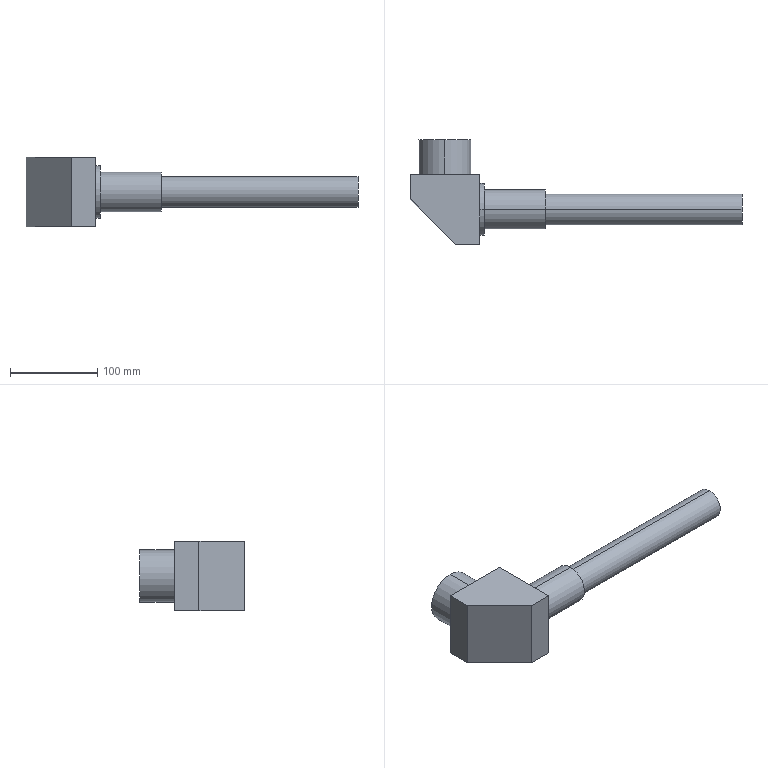Part | NX | features BREP 1 | 1 solid | 19 faces | box 380 x 120 x 80 mm | volume 858880 mm3 | plane 11 | cylinder 8 | commonest cylinder face diameters 60 x4 35 x2 45 x2
STEP:
#1=CARTESIAN_POINT('',(380.,-40.,22.5));
#2=VERTEX_POINT('',#1);
#3=CARTESIAN_POINT('',(380.,-40.,57.5));
#4=VERTEX_POINT('',#3);
#5=CARTESIAN_POINT('',(380.,-40.,40.));
#6=DIRECTION('',(1.,0.,0.));
#7=DIRECTION('',(0.,0.,-1.));
#8=AXIS2_PLACEMENT_3D('',#5,#6,#7);
#9=CIRCLE('',#8,17.5);
#10=EDGE_CURVE('',#2,#4,#9,.T.);
#11=ORIENTED_EDGE('',*,*,#10,.F.);
#12=CARTESIAN_POINT('',(155.,-40.,22.5));
#13=VERTEX_POINT('',#12);
#14=CARTESIAN_POINT('',(380.,-40.,22.5));
#15=DIRECTION('',(-1.,0.,0.));
#16=VECTOR('',#15,1000.);
#17=LINE('',#14,#16);
#18=EDGE_CURVE('',#13,#2,#17,.F.);
#19=ORIENTED_EDGE('',*,*,#18,.F.);
#20=CARTESIAN_POINT('',(155.,-40.,57.5));
#21=VERTEX_POINT('',#20);
#22=CARTESIAN_POINT('',(155.,-40.,40.));
#23=DIRECTION('',(1.,0.,0.));
#24=DIRECTION('',(0.,0.,-1.));
#25=AXIS2_PLACEMENT_3D('',#22,#23,#24);
#26=CIRCLE('',#25,17.5);
#27=EDGE_CURVE('',#13,#21,#26,.T.);
#28=ORIENTED_EDGE('',*,*,#27,.T.);
#29=CARTESIAN_POINT('',(380.,-40.,57.5));
#30=DIRECTION('',(-1.,0.,0.));
#31=VECTOR('',#30,1000.);
#32=LINE('',#29,#31);
#33=EDGE_CURVE('',#21,#4,#32,.F.);
#34=ORIENTED_EDGE('',*,*,#33,.T.);
#35=EDGE_LOOP('',(#11,#19,#28,#34));
#36=FACE_BOUND('',#35,.T.);
#37=CARTESIAN_POINT('',(380.,-40.,40.));
#38=DIRECTION('',(-1.,0.,0.));
#39=DIRECTION('',(0.,0.,1.));
#40=AXIS2_PLACEMENT_3D('',#37,#38,#39);
#41=CYLINDRICAL_SURFACE('',#40,17.5);
#42=ADVANCED_FACE('',(#36),#41,.T.);
#43=CARTESIAN_POINT('',(40.,40.,70.));
#44=VERTEX_POINT('',#43);
#45=CARTESIAN_POINT('',(40.,40.,10.));
#46=VERTEX_POINT('',#45);
#47=CARTESIAN_POINT('',(40.,40.,40.));
#48=DIRECTION('',(0.,1.,0.));
#49=DIRECTION('',(0.,0.,1.));
#50=AXIS2_PLACEMENT_3D('',#47,#48,#49);
#51=CIRCLE('',#50,30.);
#52=EDGE_CURVE('',#44,#46,#51,.T.);
#53=ORIENTED_EDGE('',*,*,#52,.F.);
#54=CARTESIAN_POINT('',(40.,0.,70.));
#55=VERTEX_POINT('',#54);
#56=CARTESIAN_POINT('',(40.,40.,70.));
#57=DIRECTION('',(0.,-1.,0.));
#58=VECTOR('',#57,1000.);
#59=LINE('',#56,#58);
#60=EDGE_CURVE('',#44,#55,#59,.T.);
#61=ORIENTED_EDGE('',*,*,#60,.T.);
#62=CARTESIAN_POINT('',(40.,0.,10.));
#63=VERTEX_POINT('',#62);
#64=CARTESIAN_POINT('',(40.,0.,40.));
#65=DIRECTION('',(0.,1.,0.));
#66=DIRECTION('',(0.,0.,1.));
#67=AXIS2_PLACEMENT_3D('',#64,#65,#66);
#68=CIRCLE('',#67,30.);
#69=EDGE_CURVE('',#55,#63,#68,.T.);
#70=ORIENTED_EDGE('',*,*,#69,.T.);
#71=CARTESIAN_POINT('',(40.,40.,10.));
#72=DIRECTION('',(0.,-1.,0.));
#73=VECTOR('',#72,1000.);
#74=LINE('',#71,#73);
#75=EDGE_CURVE('',#46,#63,#74,.T.);
#76=ORIENTED_EDGE('',*,*,#75,.F.);
#77=EDGE_LOOP('',(#53,#61,#70,#76));
#78=FACE_BOUND('',#77,.T.);
#79=CARTESIAN_POINT('',(40.,40.,40.));
#80=DIRECTION('',(0.,-1.,0.));
#81=DIRECTION('',(0.,0.,-1.));
#82=AXIS2_PLACEMENT_3D('',#79,#80,#81);
#83=CYLINDRICAL_SURFACE('',#82,30.);
#84=ADVANCED_FACE('',(#78),#83,.T.);
#85=CARTESIAN_POINT('',(155.,-40.,17.5));
#86=VERTEX_POINT('',#85);
#87=CARTESIAN_POINT('',(155.,-40.,62.5));
#88=VERTEX_POINT('',#87);
#89=CARTESIAN_POINT('',(155.,-40.,40.));
#90=DIRECTION('',(1.,0.,0.));
#91=DIRECTION('',(0.,0.,-1.));
#92=AXIS2_PLACEMENT_3D('',#89,#90,#91);
#93=CIRCLE('',#92,22.5);
#94=EDGE_CURVE('',#86,#88,#93,.T.);
#95=ORIENTED_EDGE('',*,*,#94,.F.);
#96=CARTESIAN_POINT('',(85.,-40.,17.5));
#97=VERTEX_POINT('',#96);
#98=CARTESIAN_POINT('',(155.,-40.,17.5));
#99=DIRECTION('',(-1.,0.,0.));
#100=VECTOR('',#99,1000.);
#101=LINE('',#98,#100);
#102=EDGE_CURVE('',#97,#86,#101,.F.);
#103=ORIENTED_EDGE('',*,*,#102,.F.);
#104=CARTESIAN_POINT('',(85.,-40.,62.5));
#105=VERTEX_POINT('',#104);
#106=CARTESIAN_POINT('',(85.,-40.,40.));
#107=DIRECTION('',(1.,0.,0.));
#108=DIRECTION('',(0.,0.,-1.));
#109=AXIS2_PLACEMENT_3D('',#106,#107,#108);
#110=CIRCLE('',#109,22.5);
#111=EDGE_CURVE('',#97,#105,#110,.T.);
#112=ORIENTED_EDGE('',*,*,#111,.T.);
#113=CARTESIAN_POINT('',(155.,-40.,62.5));
#114=DIRECTION('',(-1.,0.,0.));
#115=VECTOR('',#114,1000.);
#116=LINE('',#113,#115);
#117=EDGE_CURVE('',#105,#88,#116,.F.);
#118=ORIENTED_EDGE('',*,*,#117,.T.);
#119=EDGE_LOOP('',(#95,#103,#112,#118));
#120=FACE_BOUND('',#119,.T.);
#121=CARTESIAN_POINT('',(155.,-40.,40.));
#122=DIRECTION('',(-1.,0.,0.));
#123=DIRECTION('',(0.,0.,1.));
#124=AXIS2_PLACEMENT_3D('',#121,#122,#123);
#125=CYLINDRICAL_SURFACE('',#124,22.5);
#126=ADVANCED_FACE('',(#120),#125,.T.);
#127=CARTESIAN_POINT('',(85.,-40.,10.));
#128=VERTEX_POINT('',#127);
#129=CARTESIAN_POINT('',(85.,-40.,70.));
#130=VERTEX_POINT('',#129);
#131=CARTESIAN_POINT('',(85.,-40.,40.));
#132=DIRECTION('',(1.,0.,0.));
#133=DIRECTION('',(0.,0.,-1.));
#134=AXIS2_PLACEMENT_3D('',#131,#132,#133);
#135=CIRCLE('',#134,30.);
#136=EDGE_CURVE('',#128,#130,#135,.T.);
#137=ORIENTED_EDGE('',*,*,#136,.F.);
#138=CARTESIAN_POINT('',(80.,-40.,10.));
#139=VERTEX_POINT('',#138);
#140=CARTESIAN_POINT('',(85.,-40.,10.));
#141=DIRECTION('',(-1.,0.,0.));
#142=VECTOR('',#141,1000.);
#143=LINE('',#140,#142);
#144=EDGE_CURVE('',#139,#128,#143,.F.);
#145=ORIENTED_EDGE('',*,*,#144,.F.);
#146=CARTESIAN_POINT('',(80.,-40.,70.));
#147=VERTEX_POINT('',#146);
#148=CARTESIAN_POINT('',(80.,-40.,40.));
#149=DIRECTION('',(1.,0.,0.));
#150=DIRECTION('',(0.,0.,-1.));
#151=AXIS2_PLACEMENT_3D('',#148,#149,#150);
#152=CIRCLE('',#151,30.);
#153=EDGE_CURVE('',#139,#147,#152,.T.);
#154=ORIENTED_EDGE('',*,*,#153,.T.);
#155=CARTESIAN_POINT('',(85.,-40.,70.));
#156=DIRECTION('',(-1.,0.,0.));
#157=VECTOR('',#156,1000.);
#158=LINE('',#155,#157);
#159=EDGE_CURVE('',#147,#130,#158,.F.);
#160=ORIENTED_EDGE('',*,*,#159,.T.);
#161=EDGE_LOOP('',(#137,#145,#154,#160));
#162=FACE_BOUND('',#161,.T.);
#163=CARTESIAN_POINT('',(85.,-40.,40.));
#164=DIRECTION('',(-1.,0.,0.));
#165=DIRECTION('',(0.,0.,1.));
#166=AXIS2_PLACEMENT_3D('',#163,#164,#165);
#167=CYLINDRICAL_SURFACE('',#166,30.);
#168=ADVANCED_FACE('',(#162),#167,.T.);
#169=CARTESIAN_POINT('',(0.,0.,0.));
#170=VERTEX_POINT('',#169);
#171=CARTESIAN_POINT('',(0.,-28.,0.));
#172=VERTEX_POINT('',#171);
#173=CARTESIAN_POINT('',(0.,-28.,0.));
#174=DIRECTION('',(0.,-1.,0.));
#175=VECTOR('',#174,1000.);
#176=LINE('',#173,#175);
#177=EDGE_CURVE('',#170,#172,#176,.T.);
#178=ORIENTED_EDGE('',*,*,#177,.T.);
#179=CARTESIAN_POINT('',(0.,-28.,80.));
#180=VERTEX_POINT('',#179);
#181=CARTESIAN_POINT('',(0.,-28.,80.));
#182=DIRECTION('',(0.,0.,-1.));
#183=VECTOR('',#182,1000.);
#184=LINE('',#181,#183);
#185=EDGE_CURVE('',#180,#172,#184,.T.);
#186=ORIENTED_EDGE('',*,*,#185,.F.);
#187=CARTESIAN_POINT('',(0.,0.,80.));
#188=VERTEX_POINT('',#187);
#189=CARTESIAN_POINT('',(0.,-28.,80.));
#190=DIRECTION('',(0.,-1.,0.));
#191=VECTOR('',#190,1000.);
#192=LINE('',#189,#191);
#193=EDGE_CURVE('',#188,#180,#192,.T.);
#194=ORIENTED_EDGE('',*,*,#193,.F.);
#195=CARTESIAN_POINT('',(0.,0.,80.));
#196=DIRECTION('',(0.,0.,-1.));
#197=VECTOR('',#196,1000.);
#198=LINE('',#195,#197);
#199=EDGE_CURVE('',#188,#170,#198,.T.);
#200=ORIENTED_EDGE('',*,*,#199,.T.);
#201=EDGE_LOOP('',(#178,#186,#194,#200));
#202=FACE_BOUND('',#201,.T.);
#203=CARTESIAN_POINT('',(0.,-28.,80.));
#204=DIRECTION('',(1.,0.,0.));
#205=DIRECTION('',(0.,1.,0.));
#206=AXIS2_PLACEMENT_3D('',#203,#204,#205);
#207=PLANE('',#206);
#208=ADVANCED_FACE('',(#202),#207,.F.);
#209=CARTESIAN_POINT('',(52.,-80.,0.));
#210=VERTEX_POINT('',#209);
#211=CARTESIAN_POINT('',(52.,-80.,0.));
#212=DIRECTION('',(0.7071,-0.7071,0.));
#213=VECTOR('',#212,1000.);
#214=LINE('',#211,#213);
#215=EDGE_CURVE('',#172,#210,#214,.T.);
#216=ORIENTED_EDGE('',*,*,#215,.T.);
#217=CARTESIAN_POINT('',(52.,-80.,80.));
#218=VERTEX_POINT('',#217);
#219=CARTESIAN_POINT('',(52.,-80.,80.));
#220=DIRECTION('',(0.,0.,-1.));
#221=VECTOR('',#220,1000.);
#222=LINE('',#219,#221);
#223=EDGE_CURVE('',#218,#210,#222,.T.);
#224=ORIENTED_EDGE('',*,*,#223,.F.);
#225=CARTESIAN_POINT('',(52.,-80.,80.));
#226=DIRECTION('',(0.7071,-0.7071,0.));
#227=VECTOR('',#226,1000.);
#228=LINE('',#225,#227);
#229=EDGE_CURVE('',#180,#218,#228,.T.);
#230=ORIENTED_EDGE('',*,*,#229,.F.);
#231=ORIENTED_EDGE('',*,*,#185,.T.);
#232=EDGE_LOOP('',(#216,#224,#230,#231));
#233=FACE_BOUND('',#232,.T.);
#234=CARTESIAN_POINT('',(52.,-80.,80.));
#235=DIRECTION('',(0.7071,0.7071,0.));
#236=DIRECTION('',(0.,0.,-1.));
#237=AXIS2_PLACEMENT_3D('',#234,#235,#236);
#238=PLANE('',#237);
#239=ADVANCED_FACE('',(#233),#238,.F.);
#240=CARTESIAN_POINT('',(80.,-80.,0.));
#241=VERTEX_POINT('',#240);
#242=CARTESIAN_POINT('',(80.,-80.,0.));
#243=DIRECTION('',(1.,0.,0.));
#244=VECTOR('',#243,1000.);
#245=LINE('',#242,#244);
#246=EDGE_CURVE('',#210,#241,#245,.T.);
#247=ORIENTED_EDGE('',*,*,#246,.T.);
#248=CARTESIAN_POINT('',(80.,-80.,80.));
#249=VERTEX_POINT('',#248);
#250=CARTESIAN_POINT('',(80.,-80.,80.));
#251=DIRECTION('',(0.,0.,-1.));
#252=VECTOR('',#251,1000.);
#253=LINE('',#250,#252);
#254=EDGE_CURVE('',#249,#241,#253,.T.);
#255=ORIENTED_EDGE('',*,*,#254,.F.);
#256=CARTESIAN_POINT('',(80.,-80.,80.));
#257=DIRECTION('',(1.,0.,0.));
#258=VECTOR('',#257,1000.);
#259=LINE('',#256,#258);
#260=EDGE_CURVE('',#218,#249,#259,.T.);
#261=ORIENTED_EDGE('',*,*,#260,.F.);
#262=ORIENTED_EDGE('',*,*,#223,.T.);
#263=EDGE_LOOP('',(#247,#255,#261,#262));
#264=FACE_BOUND('',#263,.T.);
#265=CARTESIAN_POINT('',(80.,-80.,80.));
#266=DIRECTION('',(0.,1.,0.));
#267=DIRECTION('',(1.,0.,0.));
#268=AXIS2_PLACEMENT_3D('',#265,#266,#267);
#269=PLANE('',#268);
#270=ADVANCED_FACE('',(#264),#269,.F.);
#271=CARTESIAN_POINT('',(80.,0.,0.));
#272=VERTEX_POINT('',#271);
#273=CARTESIAN_POINT('',(80.,0.,0.));
#274=DIRECTION('',(0.,1.,0.));
#275=VECTOR('',#274,1000.);
#276=LINE('',#273,#275);
#277=EDGE_CURVE('',#241,#272,#276,.T.);
#278=ORIENTED_EDGE('',*,*,#277,.T.);
#279=CARTESIAN_POINT('',(80.,0.,80.));
#280=VERTEX_POINT('',#279);
#281=CARTESIAN_POINT('',(80.,0.,80.));
#282=DIRECTION('',(0.,0.,-1.));
#283=VECTOR('',#282,1000.);
#284=LINE('',#281,#283);
#285=EDGE_CURVE('',#280,#272,#284,.T.);
#286=ORIENTED_EDGE('',*,*,#285,.F.);
#287=CARTESIAN_POINT('',(80.,0.,80.));
#288=DIRECTION('',(0.,1.,0.));
#289=VECTOR('',#288,1000.);
#290=LINE('',#287,#289);
#291=EDGE_CURVE('',#249,#280,#290,.T.);
#292=ORIENTED_EDGE('',*,*,#291,.F.);
#293=ORIENTED_EDGE('',*,*,#254,.T.);
#294=EDGE_LOOP('',(#278,#286,#292,#293));
#295=FACE_BOUND('',#294,.T.);
#296=CARTESIAN_POINT('',(80.,-40.,40.));
#297=DIRECTION('',(1.,0.,0.));
#298=DIRECTION('',(0.,0.,-1.));
#299=AXIS2_PLACEMENT_3D('',#296,#297,#298);
#300=CIRCLE('',#299,30.);
#301=EDGE_CURVE('',#147,#139,#300,.T.);
#302=ORIENTED_EDGE('',*,*,#301,.F.);
#303=ORIENTED_EDGE('',*,*,#153,.F.);
#304=EDGE_LOOP('',(#302,#303));
#305=FACE_BOUND('',#304,.T.);
#306=CARTESIAN_POINT('',(80.,0.,80.));
#307=DIRECTION('',(-1.,0.,0.));
#308=DIRECTION('',(0.,0.,1.));
#309=AXIS2_PLACEMENT_3D('',#306,#307,#308);
#310=PLANE('',#309);
#311=ADVANCED_FACE('',(#295,#305),#310,.F.);
#312=CARTESIAN_POINT('',(0.,0.,0.));
#313=DIRECTION('',(-1.,0.,0.));
#314=VECTOR('',#313,1000.);
#315=LINE('',#312,#314);
#316=EDGE_CURVE('',#272,#170,#315,.T.);
#317=ORIENTED_EDGE('',*,*,#316,.T.);
#318=ORIENTED_EDGE('',*,*,#199,.F.);
#319=CARTESIAN_POINT('',(0.,0.,80.));
#320=DIRECTION('',(-1.,0.,0.));
#321=VECTOR('',#320,1000.);
#322=LINE('',#319,#321);
#323=EDGE_CURVE('',#280,#188,#322,.T.);
#324=ORIENTED_EDGE('',*,*,#323,.F.);
#325=ORIENTED_EDGE('',*,*,#285,.T.);
#326=EDGE_LOOP('',(#317,#318,#324,#325));
#327=FACE_BOUND('',#326,.T.);
#328=CARTESIAN_POINT('',(40.,0.,40.));
#329=DIRECTION('',(0.,1.,0.));
#330=DIRECTION('',(0.,0.,1.));
#331=AXIS2_PLACEMENT_3D('',#328,#329,#330);
#332=CIRCLE('',#331,30.);
#333=EDGE_CURVE('',#63,#55,#332,.T.);
#334=ORIENTED_EDGE('',*,*,#333,.F.);
#335=ORIENTED_EDGE('',*,*,#69,.F.);
#336=EDGE_LOOP('',(#334,#335));
#337=FACE_BOUND('',#336,.T.);
#338=CARTESIAN_POINT('',(0.,0.,80.));
#339=DIRECTION('',(0.,-1.,0.));
#340=DIRECTION('',(0.,0.,-1.));
#341=AXIS2_PLACEMENT_3D('',#338,#339,#340);
#342=PLANE('',#341);
#343=ADVANCED_FACE('',(#327,#337),#342,.F.);
#344=ORIENTED_EDGE('',*,*,#193,.T.);
#345=ORIENTED_EDGE('',*,*,#229,.T.);
#346=ORIENTED_EDGE('',*,*,#260,.T.);
#347=ORIENTED_EDGE('',*,*,#291,.T.);
#348=ORIENTED_EDGE('',*,*,#323,.T.);
#349=EDGE_LOOP('',(#344,#345,#346,#347,#348));
#350=FACE_BOUND('',#349,.T.);
#351=CARTESIAN_POINT('',(0.,0.,80.));
#352=DIRECTION('',(0.,0.,-1.));
#353=DIRECTION('',(0.,-1.,0.));
#354=AXIS2_PLACEMENT_3D('',#351,#352,#353);
#355=PLANE('',#354);
#356=ADVANCED_FACE('',(#350),#355,.F.);
#357=ORIENTED_EDGE('',*,*,#177,.F.);
#358=ORIENTED_EDGE('',*,*,#316,.F.);
#359=ORIENTED_EDGE('',*,*,#277,.F.);
#360=ORIENTED_EDGE('',*,*,#246,.F.);
#361=ORIENTED_EDGE('',*,*,#215,.F.);
#362=EDGE_LOOP('',(#357,#358,#359,#360,#361));
#363=FACE_BOUND('',#362,.T.);
#364=CARTESIAN_POINT('',(0.,0.,0.));
#365=DIRECTION('',(0.,0.,-1.));
#366=DIRECTION('',(0.,-1.,0.));
#367=AXIS2_PLACEMENT_3D('',#364,#365,#366);
#368=PLANE('',#367);
#369=ADVANCED_FACE('',(#363),#368,.T.);
#370=ORIENTED_EDGE('',*,*,#144,.T.);
#371=CARTESIAN_POINT('',(85.,-40.,40.));
#372=DIRECTION('',(1.,0.,0.));
#373=DIRECTION('',(0.,0.,-1.));
#374=AXIS2_PLACEMENT_3D('',#371,#372,#373);
#375=CIRCLE('',#374,30.);
#376=EDGE_CURVE('',#130,#128,#375,.T.);
#377=ORIENTED_EDGE('',*,*,#376,.F.);
#378=ORIENTED_EDGE('',*,*,#159,.F.);
#379=ORIENTED_EDGE('',*,*,#301,.T.);
#380=EDGE_LOOP('',(#370,#377,#378,#379));
#381=FACE_BOUND('',#380,.T.);
#382=CARTESIAN_POINT('',(85.,-40.,40.));
#383=DIRECTION('',(-1.,0.,0.));
#384=DIRECTION('',(0.,0.,1.));
#385=AXIS2_PLACEMENT_3D('',#382,#383,#384);
#386=CYLINDRICAL_SURFACE('',#385,30.);
#387=ADVANCED_FACE('',(#381),#386,.T.);
#388=ORIENTED_EDGE('',*,*,#376,.T.);
#389=ORIENTED_EDGE('',*,*,#136,.T.);
#390=EDGE_LOOP('',(#388,#389));
#391=FACE_BOUND('',#390,.T.);
#392=CARTESIAN_POINT('',(85.,-40.,40.));
#393=DIRECTION('',(1.,0.,0.));
#394=DIRECTION('',(0.,0.,-1.));
#395=AXIS2_PLACEMENT_3D('',#392,#393,#394);
#396=CIRCLE('',#395,22.5);
#397=EDGE_CURVE('',#105,#97,#396,.T.);
#398=ORIENTED_EDGE('',*,*,#397,.F.);
#399=ORIENTED_EDGE('',*,*,#111,.F.);
#400=EDGE_LOOP('',(#398,#399));
#401=FACE_BOUND('',#400,.T.);
#402=CARTESIAN_POINT('',(85.,-40.,40.));
#403=DIRECTION('',(1.,0.,0.));
#404=DIRECTION('',(0.,1.,0.));
#405=AXIS2_PLACEMENT_3D('',#402,#403,#404);
#406=PLANE('',#405);
#407=ADVANCED_FACE('',(#391,#401),#406,.T.);
#408=ORIENTED_EDGE('',*,*,#102,.T.);
#409=CARTESIAN_POINT('',(155.,-40.,40.));
#410=DIRECTION('',(1.,0.,0.));
#411=DIRECTION('',(0.,0.,-1.));
#412=AXIS2_PLACEMENT_3D('',#409,#410,#411);
#413=CIRCLE('',#412,22.5);
#414=EDGE_CURVE('',#88,#86,#413,.T.);
#415=ORIENTED_EDGE('',*,*,#414,.F.);
#416=ORIENTED_EDGE('',*,*,#117,.F.);
#417=ORIENTED_EDGE('',*,*,#397,.T.);
#418=EDGE_LOOP('',(#408,#415,#416,#417));
#419=FACE_BOUND('',#418,.T.);
#420=CARTESIAN_POINT('',(155.,-40.,40.));
#421=DIRECTION('',(-1.,0.,0.));
#422=DIRECTION('',(0.,0.,1.));
#423=AXIS2_PLACEMENT_3D('',#420,#421,#422);
#424=CYLINDRICAL_SURFACE('',#423,22.5);
#425=ADVANCED_FACE('',(#419),#424,.T.);
#426=ORIENTED_EDGE('',*,*,#414,.T.);
#427=ORIENTED_EDGE('',*,*,#94,.T.);
#428=EDGE_LOOP('',(#426,#427));
#429=FACE_BOUND('',#428,.T.);
#430=CARTESIAN_POINT('',(155.,-40.,40.));
#431=DIRECTION('',(1.,0.,0.));
#432=DIRECTION('',(0.,0.,-1.));
#433=AXIS2_PLACEMENT_3D('',#430,#431,#432);
#434=CIRCLE('',#433,17.5);
#435=EDGE_CURVE('',#21,#13,#434,.T.);
#436=ORIENTED_EDGE('',*,*,#435,.F.);
#437=ORIENTED_EDGE('',*,*,#27,.F.);
#438=EDGE_LOOP('',(#436,#437));
#439=FACE_BOUND('',#438,.T.);
#440=CARTESIAN_POINT('',(155.,-40.,40.));
#441=DIRECTION('',(1.,0.,0.));
#442=DIRECTION('',(0.,1.,0.));
#443=AXIS2_PLACEMENT_3D('',#440,#441,#442);
#444=PLANE('',#443);
#445=ADVANCED_FACE('',(#429,#439),#444,.T.);
#446=ORIENTED_EDGE('',*,*,#60,.F.);
#447=CARTESIAN_POINT('',(40.,40.,40.));
#448=DIRECTION('',(0.,1.,0.));
#449=DIRECTION('',(0.,0.,1.));
#450=AXIS2_PLACEMENT_3D('',#447,#448,#449);
#451=CIRCLE('',#450,30.);
#452=EDGE_CURVE('',#46,#44,#451,.T.);
#453=ORIENTED_EDGE('',*,*,#452,.F.);
#454=ORIENTED_EDGE('',*,*,#75,.T.);
#455=ORIENTED_EDGE('',*,*,#333,.T.);
#456=EDGE_LOOP('',(#446,#453,#454,#455));
#457=FACE_BOUND('',#456,.T.);
#458=CARTESIAN_POINT('',(40.,40.,40.));
#459=DIRECTION('',(0.,-1.,0.));
#460=DIRECTION('',(0.,0.,-1.));
#461=AXIS2_PLACEMENT_3D('',#458,#459,#460);
#462=CYLINDRICAL_SURFACE('',#461,30.);
#463=ADVANCED_FACE('',(#457),#462,.T.);
#464=ORIENTED_EDGE('',*,*,#452,.T.);
#465=ORIENTED_EDGE('',*,*,#52,.T.);
#466=EDGE_LOOP('',(#464,#465));
#467=FACE_BOUND('',#466,.T.);
#468=CARTESIAN_POINT('',(40.,40.,40.));
#469=DIRECTION('',(0.,1.,0.));
#470=DIRECTION('',(1.,0.,0.));
#471=AXIS2_PLACEMENT_3D('',#468,#469,#470);
#472=PLANE('',#471);
#473=ADVANCED_FACE('',(#467),#472,.T.);
#474=ORIENTED_EDGE('',*,*,#18,.T.);
#475=CARTESIAN_POINT('',(380.,-40.,40.));
#476=DIRECTION('',(1.,0.,0.));
#477=DIRECTION('',(0.,0.,-1.));
#478=AXIS2_PLACEMENT_3D('',#475,#476,#477);
#479=CIRCLE('',#478,17.5);
#480=EDGE_CURVE('',#4,#2,#479,.T.);
#481=ORIENTED_EDGE('',*,*,#480,.F.);
#482=ORIENTED_EDGE('',*,*,#33,.F.);
#483=ORIENTED_EDGE('',*,*,#435,.T.);
#484=EDGE_LOOP('',(#474,#481,#482,#483));
#485=FACE_BOUND('',#484,.T.);
#486=CARTESIAN_POINT('',(380.,-40.,40.));
#487=DIRECTION('',(-1.,0.,0.));
#488=DIRECTION('',(0.,0.,1.));
#489=AXIS2_PLACEMENT_3D('',#486,#487,#488);
#490=CYLINDRICAL_SURFACE('',#489,17.5);
#491=ADVANCED_FACE('',(#485),#490,.T.);
#492=ORIENTED_EDGE('',*,*,#480,.T.);
#493=ORIENTED_EDGE('',*,*,#10,.T.);
#494=EDGE_LOOP('',(#492,#493));
#495=FACE_BOUND('',#494,.T.);
#496=CARTESIAN_POINT('',(380.,-40.,40.));
#497=DIRECTION('',(1.,0.,0.));
#498=DIRECTION('',(0.,1.,0.));
#499=AXIS2_PLACEMENT_3D('',#496,#497,#498);
#500=PLANE('',#499);
#501=ADVANCED_FACE('',(#495),#500,.T.);
#502=CLOSED_SHELL('',(#42,#84,#126,#168,#208,#239,#270,#311,#343,#356,#369,#387,#407,#425,#445,#463,#473,#491,#501));
#503=MANIFOLD_SOLID_BREP('',#502);
#504=(LENGTH_UNIT()NAMED_UNIT(*)SI_UNIT(.MILLI.,.METRE.));
#505=UNCERTAINTY_MEASURE_WITH_UNIT(LENGTH_MEASURE(0.00001),#504,'','');
#506=(NAMED_UNIT(*)PLANE_ANGLE_UNIT()SI_UNIT($,.RADIAN.));
#507=(NAMED_UNIT(*)SI_UNIT($,.STERADIAN.)SOLID_ANGLE_UNIT());
#508=(GEOMETRIC_REPRESENTATION_CONTEXT(3)GLOBAL_UNCERTAINTY_ASSIGNED_CONTEXT((#505))GLOBAL_UNIT_ASSIGNED_CONTEXT((#504,#506,#507))REPRESENTATION_CONTEXT('',''));
#509=ADVANCED_BREP_SHAPE_REPRESENTATION('',(#503),#508);